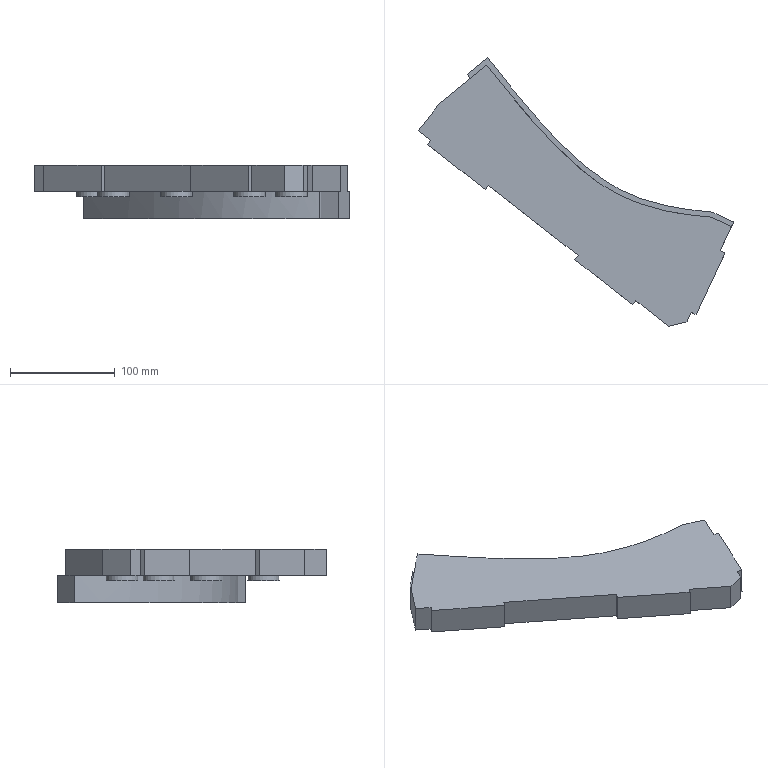Part | NX | features solid 2 | 1 solid | 35 faces | box 300.852 x 256.409 x 51 mm | volume 843468 mm3 | plane 27 | cylinder 5 | spline 3 | commonest cylinder face diameters 30 x5